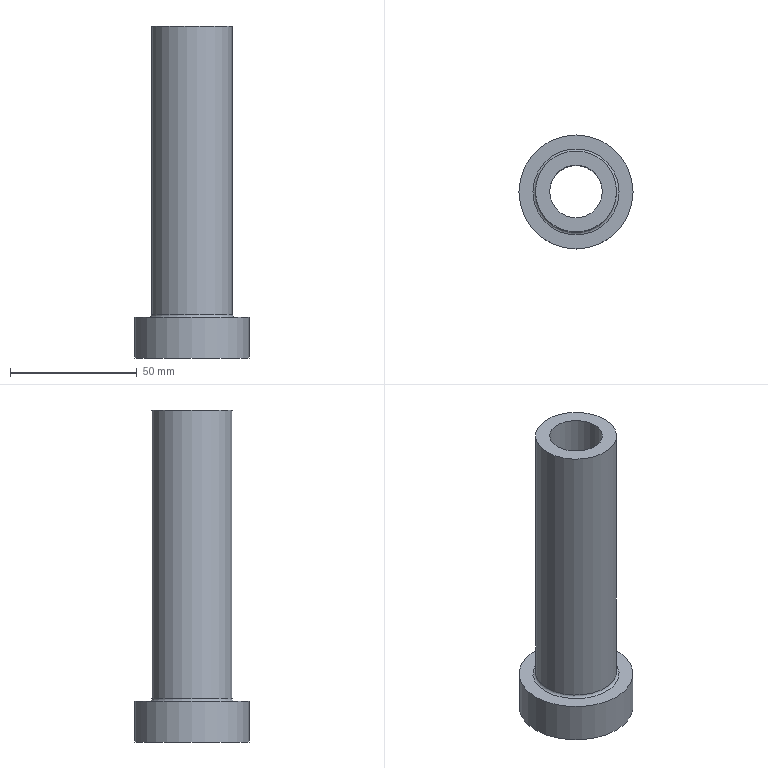Part | NX | features DT 2 | 1 solid | 7 faces | box 45 x 45 x 131 mm | volume 73444 mm3 | cylinder 3 | plane 3 | torus 1 | commonest cylinder face diameters 20.8 x1 32 x1 45 x1
STEP:
#1=CARTESIAN_POINT('',(2863.5,-627.,101.));
#2=VERTEX_POINT('',#1);
#3=CARTESIAN_POINT('',(2879.5,-627.,101.));
#4=DIRECTION('',(0.,0.,-1.));
#5=DIRECTION('',(-1.,0.,0.));
#6=AXIS2_PLACEMENT_3D('',#3,#4,#5);
#7=CIRCLE('',#6,16.);
#8=EDGE_CURVE('',#2,#2,#7,.T.);
#9=ORIENTED_EDGE('',*,*,#8,.T.);
#10=EDGE_LOOP('',(#9));
#11=FACE_BOUND('',#10,.T.);
#12=CARTESIAN_POINT('',(2863.5,-627.,-13.));
#13=VERTEX_POINT('',#12);
#14=CARTESIAN_POINT('',(2879.5,-627.,-13.));
#15=DIRECTION('',(0.,0.,1.));
#16=DIRECTION('',(1.,0.,0.));
#17=AXIS2_PLACEMENT_3D('',#14,#15,#16);
#18=CIRCLE('',#17,16.);
#19=EDGE_CURVE('',#13,#13,#18,.T.);
#20=ORIENTED_EDGE('',*,*,#19,.T.);
#21=EDGE_LOOP('',(#20));
#22=FACE_BOUND('',#21,.T.);
#23=CARTESIAN_POINT('',(2879.5,-627.,31.));
#24=DIRECTION('',(0.,0.,1.));
#25=DIRECTION('',(-1.,0.,0.));
#26=AXIS2_PLACEMENT_3D('',#23,#24,#25);
#27=CYLINDRICAL_SURFACE('',#26,16.);
#28=ADVANCED_FACE('',(#11,#22),#27,.T.);
#29=CARTESIAN_POINT('',(2869.1,-627.,-30.));
#30=VERTEX_POINT('',#29);
#31=CARTESIAN_POINT('',(2879.5,-627.,-30.));
#32=DIRECTION('',(0.,0.,-1.));
#33=DIRECTION('',(-1.,0.,0.));
#34=AXIS2_PLACEMENT_3D('',#31,#32,#33);
#35=CIRCLE('',#34,10.4);
#36=EDGE_CURVE('',#30,#30,#35,.T.);
#37=ORIENTED_EDGE('',*,*,#36,.T.);
#38=EDGE_LOOP('',(#37));
#39=FACE_BOUND('',#38,.T.);
#40=CARTESIAN_POINT('',(2869.1,-627.,101.));
#41=VERTEX_POINT('',#40);
#42=CARTESIAN_POINT('',(2879.5,-627.,101.));
#43=DIRECTION('',(0.,0.,1.));
#44=DIRECTION('',(-1.,0.,0.));
#45=AXIS2_PLACEMENT_3D('',#42,#43,#44);
#46=CIRCLE('',#45,10.4);
#47=EDGE_CURVE('',#41,#41,#46,.T.);
#48=ORIENTED_EDGE('',*,*,#47,.T.);
#49=EDGE_LOOP('',(#48));
#50=FACE_BOUND('',#49,.T.);
#51=CARTESIAN_POINT('',(2879.5,-627.,23.));
#52=DIRECTION('',(0.,0.,1.));
#53=DIRECTION('',(-1.,0.,0.));
#54=AXIS2_PLACEMENT_3D('',#51,#52,#53);
#55=CYLINDRICAL_SURFACE('',#54,10.4);
#56=ADVANCED_FACE('',(#39,#50),#55,.F.);
#57=ORIENTED_EDGE('',*,*,#19,.F.);
#58=EDGE_LOOP('',(#57));
#59=FACE_BOUND('',#58,.T.);
#60=CARTESIAN_POINT('',(2862.5,-627.,-14.));
#61=VERTEX_POINT('',#60);
#62=CARTESIAN_POINT('',(2879.5,-627.,-14.));
#63=DIRECTION('',(0.,0.,-1.));
#64=DIRECTION('',(1.,0.,0.));
#65=AXIS2_PLACEMENT_3D('',#62,#63,#64);
#66=CIRCLE('',#65,17.);
#67=EDGE_CURVE('',#61,#61,#66,.T.);
#68=ORIENTED_EDGE('',*,*,#67,.F.);
#69=EDGE_LOOP('',(#68));
#70=FACE_BOUND('',#69,.T.);
#71=CARTESIAN_POINT('',(2879.5,-627.,-13.));
#72=DIRECTION('',(0.,0.,-1.));
#73=DIRECTION('',(1.,0.,0.));
#74=AXIS2_PLACEMENT_3D('',#71,#72,#73);
#75=TOROIDAL_SURFACE('',#74,17.,1.);
#76=ADVANCED_FACE('',(#59,#70),#75,.F.);
#77=CARTESIAN_POINT('',(2857.,-627.,-14.));
#78=VERTEX_POINT('',#77);
#79=CARTESIAN_POINT('',(2879.5,-627.,-14.));
#80=DIRECTION('',(0.,0.,-1.));
#81=DIRECTION('',(-1.,0.,0.));
#82=AXIS2_PLACEMENT_3D('',#79,#80,#81);
#83=CIRCLE('',#82,22.5);
#84=EDGE_CURVE('',#78,#78,#83,.T.);
#85=ORIENTED_EDGE('',*,*,#84,.F.);
#86=EDGE_LOOP('',(#85));
#87=FACE_BOUND('',#86,.T.);
#88=ORIENTED_EDGE('',*,*,#67,.T.);
#89=EDGE_LOOP('',(#88));
#90=FACE_BOUND('',#89,.T.);
#91=CARTESIAN_POINT('',(2879.5,-627.,-14.));
#92=DIRECTION('',(0.,0.,1.));
#93=DIRECTION('',(-1.,0.,0.));
#94=AXIS2_PLACEMENT_3D('',#91,#92,#93);
#95=PLANE('',#94);
#96=ADVANCED_FACE('',(#87,#90),#95,.T.);
#97=ORIENTED_EDGE('',*,*,#47,.F.);
#98=EDGE_LOOP('',(#97));
#99=FACE_BOUND('',#98,.T.);
#100=ORIENTED_EDGE('',*,*,#8,.F.);
#101=EDGE_LOOP('',(#100));
#102=FACE_BOUND('',#101,.T.);
#103=CARTESIAN_POINT('',(2879.5,-627.,101.));
#104=DIRECTION('',(0.,0.,1.));
#105=DIRECTION('',(-1.,0.,0.));
#106=AXIS2_PLACEMENT_3D('',#103,#104,#105);
#107=PLANE('',#106);
#108=ADVANCED_FACE('',(#99,#102),#107,.T.);
#109=CARTESIAN_POINT('',(2857.,-627.,-30.));
#110=VERTEX_POINT('',#109);
#111=CARTESIAN_POINT('',(2879.5,-627.,-30.));
#112=DIRECTION('',(0.,0.,1.));
#113=DIRECTION('',(-1.,0.,0.));
#114=AXIS2_PLACEMENT_3D('',#111,#112,#113);
#115=CIRCLE('',#114,22.5);
#116=EDGE_CURVE('',#110,#110,#115,.T.);
#117=ORIENTED_EDGE('',*,*,#116,.T.);
#118=EDGE_LOOP('',(#117));
#119=FACE_BOUND('',#118,.T.);
#120=ORIENTED_EDGE('',*,*,#84,.T.);
#121=EDGE_LOOP('',(#120));
#122=FACE_BOUND('',#121,.T.);
#123=CARTESIAN_POINT('',(2879.5,-627.,-22.));
#124=DIRECTION('',(0.,0.,1.));
#125=DIRECTION('',(-1.,0.,0.));
#126=AXIS2_PLACEMENT_3D('',#123,#124,#125);
#127=CYLINDRICAL_SURFACE('',#126,22.5);
#128=ADVANCED_FACE('',(#119,#122),#127,.T.);
#129=ORIENTED_EDGE('',*,*,#36,.F.);
#130=EDGE_LOOP('',(#129));
#131=FACE_BOUND('',#130,.T.);
#132=ORIENTED_EDGE('',*,*,#116,.F.);
#133=EDGE_LOOP('',(#132));
#134=FACE_BOUND('',#133,.T.);
#135=CARTESIAN_POINT('',(2879.5,-627.,-30.));
#136=DIRECTION('',(0.,0.,-1.));
#137=DIRECTION('',(1.,0.,0.));
#138=AXIS2_PLACEMENT_3D('',#135,#136,#137);
#139=PLANE('',#138);
#140=ADVANCED_FACE('',(#131,#134),#139,.T.);
#141=CLOSED_SHELL('',(#28,#56,#76,#96,#108,#128,#140));
#142=MANIFOLD_SOLID_BREP('',#141);
#143=(LENGTH_UNIT()NAMED_UNIT(*)SI_UNIT(.MILLI.,.METRE.));
#144=UNCERTAINTY_MEASURE_WITH_UNIT(LENGTH_MEASURE(0.00001),#143,'','');
#145=(NAMED_UNIT(*)PLANE_ANGLE_UNIT()SI_UNIT($,.RADIAN.));
#146=(NAMED_UNIT(*)SI_UNIT($,.STERADIAN.)SOLID_ANGLE_UNIT());
#147=(GEOMETRIC_REPRESENTATION_CONTEXT(3)GLOBAL_UNCERTAINTY_ASSIGNED_CONTEXT((#144))GLOBAL_UNIT_ASSIGNED_CONTEXT((#143,#145,#146))REPRESENTATION_CONTEXT('',''));
#148=ADVANCED_BREP_SHAPE_REPRESENTATION('',(#142),#147);